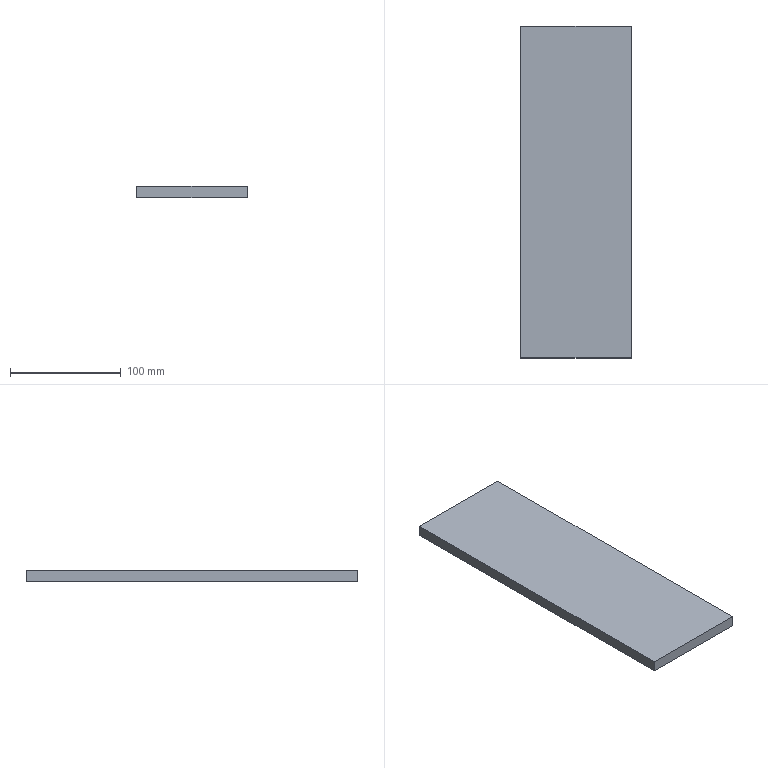Part | STEP file | Frame_top | 1 solid | 6 faces | box 100 x 300 x 10 mm | volume 300000 mm3 | plane 6
STEP:
#1=CARTESIAN_POINT('',(0.,0.,0.));
#2=DIRECTION('',(0.,0.,1.));
#3=DIRECTION('',(1.,0.,0.));
#4=AXIS2_PLACEMENT_3D('',#1,#2,#3);
#5=CARTESIAN_POINT('',(-50.,150.,0.));
#6=VERTEX_POINT('',#5);
#7=CARTESIAN_POINT('',(-50.,150.,-10.));
#8=VERTEX_POINT('',#7);
#9=CARTESIAN_POINT('',(-50.,150.,0.));
#10=DIRECTION('',(0.,0.,-1.));
#11=VECTOR('',#10,1.);
#12=LINE('',#9,#11);
#13=CARTESIAN_POINT('',(-50.,150.,0.));
#14=DIRECTION('',(-1.,0.,0.));
#15=DIRECTION('',(0.,-1.,0.));
#16=AXIS2_PLACEMENT_3D('',#13,#14,#15);
#17=PLANE('',#16);
#18=CARTESIAN_POINT('',(0.,0.));
#19=DIRECTION('',(0.,-1.));
#20=VECTOR('',#19,1.);
#21=LINE('',#18,#20);
#22=(GEOMETRIC_REPRESENTATION_CONTEXT(2)PARAMETRIC_REPRESENTATION_CONTEXT()REPRESENTATION_CONTEXT('',''));
#23=DEFINITIONAL_REPRESENTATION('',(#21),#22);
#24=PCURVE('',#17,#23);
#25=CARTESIAN_POINT('',(50.,150.,0.));
#26=DIRECTION('',(0.,1.,0.));
#27=DIRECTION('',(-1.,0.,0.));
#28=AXIS2_PLACEMENT_3D('',#25,#26,#27);
#29=PLANE('',#28);
#30=CARTESIAN_POINT('',(100.,0.));
#31=DIRECTION('',(0.,-1.));
#32=VECTOR('',#31,1.);
#33=LINE('',#30,#32);
#34=(GEOMETRIC_REPRESENTATION_CONTEXT(2)PARAMETRIC_REPRESENTATION_CONTEXT()REPRESENTATION_CONTEXT('',''));
#35=DEFINITIONAL_REPRESENTATION('',(#33),#34);
#36=PCURVE('',#29,#35);
#37=SURFACE_CURVE('',#12,(#24,#36),.PCURVE_S1.);
#38=EDGE_CURVE('',#6,#8,#37,.T.);
#39=ORIENTED_EDGE('',*,*,#38,.T.);
#40=CARTESIAN_POINT('',(-50.,-150.,-10.));
#41=VERTEX_POINT('',#40);
#42=CARTESIAN_POINT('',(-50.,150.,-10.));
#43=DIRECTION('',(0.,-1.,0.));
#44=VECTOR('',#43,1.);
#45=LINE('',#42,#44);
#46=CARTESIAN_POINT('',(0.,-10.));
#47=DIRECTION('',(1.,0.));
#48=VECTOR('',#47,1.);
#49=LINE('',#46,#48);
#50=(GEOMETRIC_REPRESENTATION_CONTEXT(2)PARAMETRIC_REPRESENTATION_CONTEXT()REPRESENTATION_CONTEXT('',''));
#51=DEFINITIONAL_REPRESENTATION('',(#49),#50);
#52=PCURVE('',#17,#51);
#53=CARTESIAN_POINT('',(0.,0.,-10.));
#54=DIRECTION('',(0.,0.,1.));
#55=DIRECTION('',(1.,0.,0.));
#56=AXIS2_PLACEMENT_3D('',#53,#54,#55);
#57=PLANE('',#56);
#58=CARTESIAN_POINT('',(-50.,150.));
#59=DIRECTION('',(0.,-1.));
#60=VECTOR('',#59,1.);
#61=LINE('',#58,#60);
#62=(GEOMETRIC_REPRESENTATION_CONTEXT(2)PARAMETRIC_REPRESENTATION_CONTEXT()REPRESENTATION_CONTEXT('',''));
#63=DEFINITIONAL_REPRESENTATION('',(#61),#62);
#64=PCURVE('',#57,#63);
#65=SURFACE_CURVE('',#45,(#52,#64),.PCURVE_S1.);
#66=EDGE_CURVE('',#8,#41,#65,.T.);
#67=ORIENTED_EDGE('',*,*,#66,.T.);
#68=CARTESIAN_POINT('',(-50.,-150.,0.));
#69=VERTEX_POINT('',#68);
#70=CARTESIAN_POINT('',(-50.,-150.,0.));
#71=DIRECTION('',(0.,0.,-1.));
#72=VECTOR('',#71,1.);
#73=LINE('',#70,#72);
#74=CARTESIAN_POINT('',(300.,0.));
#75=DIRECTION('',(0.,-1.));
#76=VECTOR('',#75,1.);
#77=LINE('',#74,#76);
#78=(GEOMETRIC_REPRESENTATION_CONTEXT(2)PARAMETRIC_REPRESENTATION_CONTEXT()REPRESENTATION_CONTEXT('',''));
#79=DEFINITIONAL_REPRESENTATION('',(#77),#78);
#80=PCURVE('',#17,#79);
#81=CARTESIAN_POINT('',(-50.,-150.,0.));
#82=DIRECTION('',(0.,-1.,0.));
#83=DIRECTION('',(1.,0.,0.));
#84=AXIS2_PLACEMENT_3D('',#81,#82,#83);
#85=PLANE('',#84);
#86=CARTESIAN_POINT('',(0.,0.));
#87=DIRECTION('',(0.,-1.));
#88=VECTOR('',#87,1.);
#89=LINE('',#86,#88);
#90=(GEOMETRIC_REPRESENTATION_CONTEXT(2)PARAMETRIC_REPRESENTATION_CONTEXT()REPRESENTATION_CONTEXT('',''));
#91=DEFINITIONAL_REPRESENTATION('',(#89),#90);
#92=PCURVE('',#85,#91);
#93=SURFACE_CURVE('',#73,(#80,#92),.PCURVE_S1.);
#94=EDGE_CURVE('',#69,#41,#93,.T.);
#95=ORIENTED_EDGE('',*,*,#94,.F.);
#96=CARTESIAN_POINT('',(-50.,150.,0.));
#97=DIRECTION('',(0.,-1.,0.));
#98=VECTOR('',#97,1.);
#99=LINE('',#96,#98);
#100=CARTESIAN_POINT('',(0.,0.));
#101=DIRECTION('',(1.,0.));
#102=VECTOR('',#101,1.);
#103=LINE('',#100,#102);
#104=(GEOMETRIC_REPRESENTATION_CONTEXT(2)PARAMETRIC_REPRESENTATION_CONTEXT()REPRESENTATION_CONTEXT('',''));
#105=DEFINITIONAL_REPRESENTATION('',(#103),#104);
#106=PCURVE('',#17,#105);
#107=CARTESIAN_POINT('',(0.,0.,0.));
#108=DIRECTION('',(0.,0.,1.));
#109=DIRECTION('',(1.,0.,0.));
#110=AXIS2_PLACEMENT_3D('',#107,#108,#109);
#111=PLANE('',#110);
#112=CARTESIAN_POINT('',(-50.,150.));
#113=DIRECTION('',(0.,-1.));
#114=VECTOR('',#113,1.);
#115=LINE('',#112,#114);
#116=(GEOMETRIC_REPRESENTATION_CONTEXT(2)PARAMETRIC_REPRESENTATION_CONTEXT()REPRESENTATION_CONTEXT('',''));
#117=DEFINITIONAL_REPRESENTATION('',(#115),#116);
#118=PCURVE('',#111,#117);
#119=SURFACE_CURVE('',#99,(#106,#118),.PCURVE_S1.);
#120=EDGE_CURVE('',#6,#69,#119,.T.);
#121=ORIENTED_EDGE('',*,*,#120,.F.);
#122=EDGE_LOOP('',(#39,#67,#95,#121));
#123=FACE_BOUND('',#122,.T.);
#124=ADVANCED_FACE('',(#123),#17,.T.);
#125=ORIENTED_EDGE('',*,*,#94,.T.);
#126=CARTESIAN_POINT('',(50.,-150.,-10.));
#127=VERTEX_POINT('',#126);
#128=CARTESIAN_POINT('',(-50.,-150.,-10.));
#129=DIRECTION('',(1.,0.,0.));
#130=VECTOR('',#129,1.);
#131=LINE('',#128,#130);
#132=CARTESIAN_POINT('',(0.,-10.));
#133=DIRECTION('',(1.,0.));
#134=VECTOR('',#133,1.);
#135=LINE('',#132,#134);
#136=(GEOMETRIC_REPRESENTATION_CONTEXT(2)PARAMETRIC_REPRESENTATION_CONTEXT()REPRESENTATION_CONTEXT('',''));
#137=DEFINITIONAL_REPRESENTATION('',(#135),#136);
#138=PCURVE('',#85,#137);
#139=CARTESIAN_POINT('',(-50.,-150.));
#140=DIRECTION('',(1.,0.));
#141=VECTOR('',#140,1.);
#142=LINE('',#139,#141);
#143=(GEOMETRIC_REPRESENTATION_CONTEXT(2)PARAMETRIC_REPRESENTATION_CONTEXT()REPRESENTATION_CONTEXT('',''));
#144=DEFINITIONAL_REPRESENTATION('',(#142),#143);
#145=PCURVE('',#57,#144);
#146=SURFACE_CURVE('',#131,(#138,#145),.PCURVE_S1.);
#147=EDGE_CURVE('',#41,#127,#146,.T.);
#148=ORIENTED_EDGE('',*,*,#147,.T.);
#149=CARTESIAN_POINT('',(50.,-150.,0.));
#150=VERTEX_POINT('',#149);
#151=CARTESIAN_POINT('',(50.,-150.,0.));
#152=DIRECTION('',(0.,0.,-1.));
#153=VECTOR('',#152,1.);
#154=LINE('',#151,#153);
#155=CARTESIAN_POINT('',(100.,0.));
#156=DIRECTION('',(0.,-1.));
#157=VECTOR('',#156,1.);
#158=LINE('',#155,#157);
#159=(GEOMETRIC_REPRESENTATION_CONTEXT(2)PARAMETRIC_REPRESENTATION_CONTEXT()REPRESENTATION_CONTEXT('',''));
#160=DEFINITIONAL_REPRESENTATION('',(#158),#159);
#161=PCURVE('',#85,#160);
#162=CARTESIAN_POINT('',(50.,-150.,0.));
#163=DIRECTION('',(1.,0.,0.));
#164=DIRECTION('',(0.,1.,0.));
#165=AXIS2_PLACEMENT_3D('',#162,#163,#164);
#166=PLANE('',#165);
#167=CARTESIAN_POINT('',(0.,0.));
#168=DIRECTION('',(0.,-1.));
#169=VECTOR('',#168,1.);
#170=LINE('',#167,#169);
#171=(GEOMETRIC_REPRESENTATION_CONTEXT(2)PARAMETRIC_REPRESENTATION_CONTEXT()REPRESENTATION_CONTEXT('',''));
#172=DEFINITIONAL_REPRESENTATION('',(#170),#171);
#173=PCURVE('',#166,#172);
#174=SURFACE_CURVE('',#154,(#161,#173),.PCURVE_S1.);
#175=EDGE_CURVE('',#150,#127,#174,.T.);
#176=ORIENTED_EDGE('',*,*,#175,.F.);
#177=CARTESIAN_POINT('',(-50.,-150.,0.));
#178=DIRECTION('',(1.,0.,0.));
#179=VECTOR('',#178,1.);
#180=LINE('',#177,#179);
#181=CARTESIAN_POINT('',(0.,0.));
#182=DIRECTION('',(1.,0.));
#183=VECTOR('',#182,1.);
#184=LINE('',#181,#183);
#185=(GEOMETRIC_REPRESENTATION_CONTEXT(2)PARAMETRIC_REPRESENTATION_CONTEXT()REPRESENTATION_CONTEXT('',''));
#186=DEFINITIONAL_REPRESENTATION('',(#184),#185);
#187=PCURVE('',#85,#186);
#188=CARTESIAN_POINT('',(-50.,-150.));
#189=DIRECTION('',(1.,0.));
#190=VECTOR('',#189,1.);
#191=LINE('',#188,#190);
#192=(GEOMETRIC_REPRESENTATION_CONTEXT(2)PARAMETRIC_REPRESENTATION_CONTEXT()REPRESENTATION_CONTEXT('',''));
#193=DEFINITIONAL_REPRESENTATION('',(#191),#192);
#194=PCURVE('',#111,#193);
#195=SURFACE_CURVE('',#180,(#187,#194),.PCURVE_S1.);
#196=EDGE_CURVE('',#69,#150,#195,.T.);
#197=ORIENTED_EDGE('',*,*,#196,.F.);
#198=EDGE_LOOP('',(#125,#148,#176,#197));
#199=FACE_BOUND('',#198,.T.);
#200=ADVANCED_FACE('',(#199),#85,.T.);
#201=ORIENTED_EDGE('',*,*,#175,.T.);
#202=CARTESIAN_POINT('',(50.,150.,-10.));
#203=VERTEX_POINT('',#202);
#204=CARTESIAN_POINT('',(50.,-150.,-10.));
#205=DIRECTION('',(0.,1.,0.));
#206=VECTOR('',#205,1.);
#207=LINE('',#204,#206);
#208=CARTESIAN_POINT('',(0.,-10.));
#209=DIRECTION('',(1.,0.));
#210=VECTOR('',#209,1.);
#211=LINE('',#208,#210);
#212=(GEOMETRIC_REPRESENTATION_CONTEXT(2)PARAMETRIC_REPRESENTATION_CONTEXT()REPRESENTATION_CONTEXT('',''));
#213=DEFINITIONAL_REPRESENTATION('',(#211),#212);
#214=PCURVE('',#166,#213);
#215=CARTESIAN_POINT('',(50.,-150.));
#216=DIRECTION('',(0.,1.));
#217=VECTOR('',#216,1.);
#218=LINE('',#215,#217);
#219=(GEOMETRIC_REPRESENTATION_CONTEXT(2)PARAMETRIC_REPRESENTATION_CONTEXT()REPRESENTATION_CONTEXT('',''));
#220=DEFINITIONAL_REPRESENTATION('',(#218),#219);
#221=PCURVE('',#57,#220);
#222=SURFACE_CURVE('',#207,(#214,#221),.PCURVE_S1.);
#223=EDGE_CURVE('',#127,#203,#222,.T.);
#224=ORIENTED_EDGE('',*,*,#223,.T.);
#225=CARTESIAN_POINT('',(50.,150.,0.));
#226=VERTEX_POINT('',#225);
#227=CARTESIAN_POINT('',(50.,150.,0.));
#228=DIRECTION('',(0.,0.,-1.));
#229=VECTOR('',#228,1.);
#230=LINE('',#227,#229);
#231=CARTESIAN_POINT('',(300.,0.));
#232=DIRECTION('',(0.,-1.));
#233=VECTOR('',#232,1.);
#234=LINE('',#231,#233);
#235=(GEOMETRIC_REPRESENTATION_CONTEXT(2)PARAMETRIC_REPRESENTATION_CONTEXT()REPRESENTATION_CONTEXT('',''));
#236=DEFINITIONAL_REPRESENTATION('',(#234),#235);
#237=PCURVE('',#166,#236);
#238=CARTESIAN_POINT('',(0.,0.));
#239=DIRECTION('',(0.,-1.));
#240=VECTOR('',#239,1.);
#241=LINE('',#238,#240);
#242=(GEOMETRIC_REPRESENTATION_CONTEXT(2)PARAMETRIC_REPRESENTATION_CONTEXT()REPRESENTATION_CONTEXT('',''));
#243=DEFINITIONAL_REPRESENTATION('',(#241),#242);
#244=PCURVE('',#29,#243);
#245=SURFACE_CURVE('',#230,(#237,#244),.PCURVE_S1.);
#246=EDGE_CURVE('',#226,#203,#245,.T.);
#247=ORIENTED_EDGE('',*,*,#246,.F.);
#248=CARTESIAN_POINT('',(50.,-150.,0.));
#249=DIRECTION('',(0.,1.,0.));
#250=VECTOR('',#249,1.);
#251=LINE('',#248,#250);
#252=CARTESIAN_POINT('',(0.,0.));
#253=DIRECTION('',(1.,0.));
#254=VECTOR('',#253,1.);
#255=LINE('',#252,#254);
#256=(GEOMETRIC_REPRESENTATION_CONTEXT(2)PARAMETRIC_REPRESENTATION_CONTEXT()REPRESENTATION_CONTEXT('',''));
#257=DEFINITIONAL_REPRESENTATION('',(#255),#256);
#258=PCURVE('',#166,#257);
#259=CARTESIAN_POINT('',(50.,-150.));
#260=DIRECTION('',(0.,1.));
#261=VECTOR('',#260,1.);
#262=LINE('',#259,#261);
#263=(GEOMETRIC_REPRESENTATION_CONTEXT(2)PARAMETRIC_REPRESENTATION_CONTEXT()REPRESENTATION_CONTEXT('',''));
#264=DEFINITIONAL_REPRESENTATION('',(#262),#263);
#265=PCURVE('',#111,#264);
#266=SURFACE_CURVE('',#251,(#258,#265),.PCURVE_S1.);
#267=EDGE_CURVE('',#150,#226,#266,.T.);
#268=ORIENTED_EDGE('',*,*,#267,.F.);
#269=EDGE_LOOP('',(#201,#224,#247,#268));
#270=FACE_BOUND('',#269,.T.);
#271=ADVANCED_FACE('',(#270),#166,.T.);
#272=ORIENTED_EDGE('',*,*,#246,.T.);
#273=CARTESIAN_POINT('',(50.,150.,-10.));
#274=DIRECTION('',(-1.,0.,0.));
#275=VECTOR('',#274,1.);
#276=LINE('',#273,#275);
#277=CARTESIAN_POINT('',(0.,-10.));
#278=DIRECTION('',(1.,0.));
#279=VECTOR('',#278,1.);
#280=LINE('',#277,#279);
#281=(GEOMETRIC_REPRESENTATION_CONTEXT(2)PARAMETRIC_REPRESENTATION_CONTEXT()REPRESENTATION_CONTEXT('',''));
#282=DEFINITIONAL_REPRESENTATION('',(#280),#281);
#283=PCURVE('',#29,#282);
#284=CARTESIAN_POINT('',(50.,150.));
#285=DIRECTION('',(-1.,0.));
#286=VECTOR('',#285,1.);
#287=LINE('',#284,#286);
#288=(GEOMETRIC_REPRESENTATION_CONTEXT(2)PARAMETRIC_REPRESENTATION_CONTEXT()REPRESENTATION_CONTEXT('',''));
#289=DEFINITIONAL_REPRESENTATION('',(#287),#288);
#290=PCURVE('',#57,#289);
#291=SURFACE_CURVE('',#276,(#283,#290),.PCURVE_S1.);
#292=EDGE_CURVE('',#203,#8,#291,.T.);
#293=ORIENTED_EDGE('',*,*,#292,.T.);
#294=ORIENTED_EDGE('',*,*,#38,.F.);
#295=CARTESIAN_POINT('',(50.,150.,0.));
#296=DIRECTION('',(-1.,0.,0.));
#297=VECTOR('',#296,1.);
#298=LINE('',#295,#297);
#299=CARTESIAN_POINT('',(0.,0.));
#300=DIRECTION('',(1.,0.));
#301=VECTOR('',#300,1.);
#302=LINE('',#299,#301);
#303=(GEOMETRIC_REPRESENTATION_CONTEXT(2)PARAMETRIC_REPRESENTATION_CONTEXT()REPRESENTATION_CONTEXT('',''));
#304=DEFINITIONAL_REPRESENTATION('',(#302),#303);
#305=PCURVE('',#29,#304);
#306=CARTESIAN_POINT('',(50.,150.));
#307=DIRECTION('',(-1.,0.));
#308=VECTOR('',#307,1.);
#309=LINE('',#306,#308);
#310=(GEOMETRIC_REPRESENTATION_CONTEXT(2)PARAMETRIC_REPRESENTATION_CONTEXT()REPRESENTATION_CONTEXT('',''));
#311=DEFINITIONAL_REPRESENTATION('',(#309),#310);
#312=PCURVE('',#111,#311);
#313=SURFACE_CURVE('',#298,(#305,#312),.PCURVE_S1.);
#314=EDGE_CURVE('',#226,#6,#313,.T.);
#315=ORIENTED_EDGE('',*,*,#314,.F.);
#316=EDGE_LOOP('',(#272,#293,#294,#315));
#317=FACE_BOUND('',#316,.T.);
#318=ADVANCED_FACE('',(#317),#29,.T.);
#319=ORIENTED_EDGE('',*,*,#120,.T.);
#320=ORIENTED_EDGE('',*,*,#196,.T.);
#321=ORIENTED_EDGE('',*,*,#267,.T.);
#322=ORIENTED_EDGE('',*,*,#314,.T.);
#323=EDGE_LOOP('',(#319,#320,#321,#322));
#324=FACE_BOUND('',#323,.T.);
#325=ADVANCED_FACE('',(#324),#111,.T.);
#326=ORIENTED_EDGE('',*,*,#66,.T.);
#327=ORIENTED_EDGE('',*,*,#147,.T.);
#328=ORIENTED_EDGE('',*,*,#223,.T.);
#329=ORIENTED_EDGE('',*,*,#292,.T.);
#330=EDGE_LOOP('',(#326,#327,#328,#329));
#331=FACE_BOUND('',#330,.F.);
#332=ADVANCED_FACE('',(#331),#57,.F.);
#333=CLOSED_SHELL('',(#124,#200,#271,#318,#325,#332));
#334=MANIFOLD_SOLID_BREP('',#333);
#335=(LENGTH_UNIT()NAMED_UNIT(*)SI_UNIT(.MILLI.,.METRE.));
#336=UNCERTAINTY_MEASURE_WITH_UNIT(LENGTH_MEASURE(0.0000001),#335,'','');
#337=(NAMED_UNIT(*)PLANE_ANGLE_UNIT()SI_UNIT($,.RADIAN.));
#338=(NAMED_UNIT(*)SI_UNIT($,.STERADIAN.)SOLID_ANGLE_UNIT());
#339=(GEOMETRIC_REPRESENTATION_CONTEXT(3)GLOBAL_UNCERTAINTY_ASSIGNED_CONTEXT((#336))GLOBAL_UNIT_ASSIGNED_CONTEXT((#335,#337,#338))REPRESENTATION_CONTEXT('',''));
#340=ADVANCED_BREP_SHAPE_REPRESENTATION('',(#4,#334),#339);